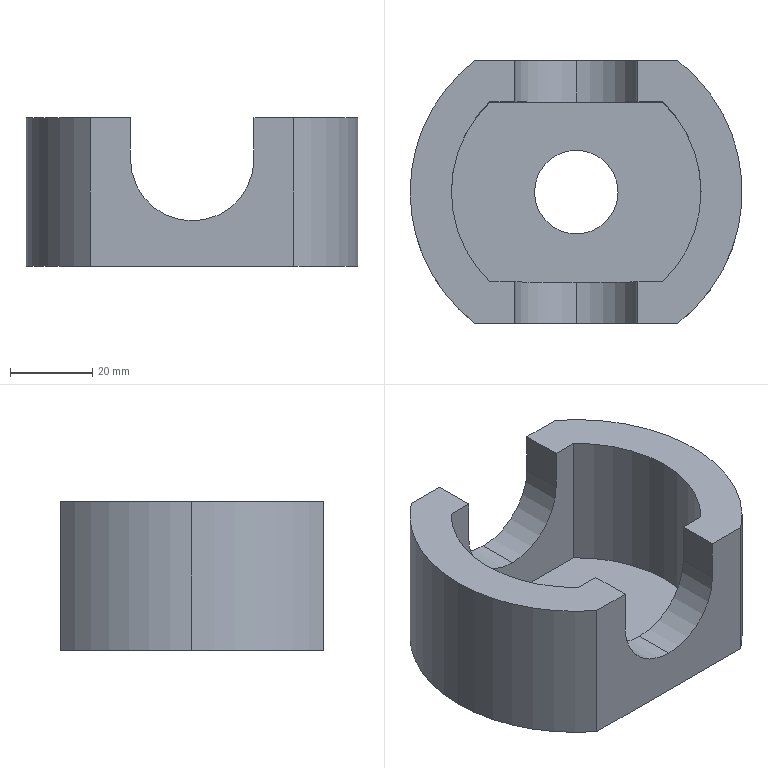Part | SolidWorks | features BaseBody 1 | 1 solid | 24 faces | box 80.6 x 63.7 x 36 mm | volume 68001 mm3 | cylinder 12 | plane 12 | commonest cylinder face diameters 30 x4 60.6 x3 80.6 x3 20.3 x2
STEP:
#1=CARTESIAN_POINT('',(2.562,-19.084,26.));
#2=VERTEX_POINT('',#1);
#3=CARTESIAN_POINT('',(-12.438,-19.084,11.));
#4=VERTEX_POINT('',#3);
#5=CARTESIAN_POINT('',(-12.438,-19.084,26.));
#6=DIRECTION('',(0.,1.,0.));
#7=DIRECTION('',(0.,0.,1.));
#8=AXIS2_PLACEMENT_3D('',#5,#6,#7);
#9=CIRCLE('',#8,15.);
#10=EDGE_CURVE('',#2,#4,#9,.T.);
#11=ORIENTED_EDGE('',*,*,#10,.T.);
#12=CARTESIAN_POINT('',(-12.438,-29.084,11.));
#13=VERTEX_POINT('',#12);
#14=CARTESIAN_POINT('',(-12.438,34.616,11.));
#15=DIRECTION('',(0.,-1.,0.));
#16=VECTOR('',#15,1000.);
#17=LINE('',#14,#16);
#18=EDGE_CURVE('',#4,#13,#17,.T.);
#19=ORIENTED_EDGE('',*,*,#18,.T.);
#20=CARTESIAN_POINT('',(2.562,-29.084,26.));
#21=VERTEX_POINT('',#20);
#22=CARTESIAN_POINT('',(-12.438,-29.084,26.));
#23=DIRECTION('',(0.,-1.,0.));
#24=DIRECTION('',(0.,0.,-1.));
#25=AXIS2_PLACEMENT_3D('',#22,#23,#24);
#26=CIRCLE('',#25,15.);
#27=EDGE_CURVE('',#13,#21,#26,.T.);
#28=ORIENTED_EDGE('',*,*,#27,.T.);
#29=CARTESIAN_POINT('',(2.562,34.616,26.));
#30=DIRECTION('',(0.,-1.,0.));
#31=VECTOR('',#30,1000.);
#32=LINE('',#29,#31);
#33=EDGE_CURVE('',#2,#21,#32,.T.);
#34=ORIENTED_EDGE('',*,*,#33,.F.);
#35=EDGE_LOOP('',(#11,#19,#28,#34));
#36=FACE_OUTER_BOUND('',#35,.T.);
#37=CARTESIAN_POINT('',(-12.438,34.616,26.));
#38=DIRECTION('',(0.,-1.,0.));
#39=DIRECTION('',(0.,0.,-1.));
#40=AXIS2_PLACEMENT_3D('',#37,#38,#39);
#41=CYLINDRICAL_SURFACE('',#40,15.);
#42=ADVANCED_FACE('',(#36),#41,.F.);
#43=CARTESIAN_POINT('',(-12.438,34.616,11.));
#44=VERTEX_POINT('',#43);
#45=CARTESIAN_POINT('',(2.562,34.616,26.));
#46=VERTEX_POINT('',#45);
#47=CARTESIAN_POINT('',(-12.438,34.616,26.));
#48=DIRECTION('',(0.,-1.,0.));
#49=DIRECTION('',(0.,0.,-1.));
#50=AXIS2_PLACEMENT_3D('',#47,#48,#49);
#51=CIRCLE('',#50,15.);
#52=EDGE_CURVE('',#44,#46,#51,.T.);
#53=ORIENTED_EDGE('',*,*,#52,.F.);
#54=CARTESIAN_POINT('',(-12.438,24.616,11.));
#55=VERTEX_POINT('',#54);
#56=CARTESIAN_POINT('',(-12.438,34.616,11.));
#57=DIRECTION('',(0.,-1.,0.));
#58=VECTOR('',#57,1000.);
#59=LINE('',#56,#58);
#60=EDGE_CURVE('',#44,#55,#59,.T.);
#61=ORIENTED_EDGE('',*,*,#60,.T.);
#62=CARTESIAN_POINT('',(2.562,24.616,26.));
#63=VERTEX_POINT('',#62);
#64=CARTESIAN_POINT('',(-12.438,24.616,26.));
#65=DIRECTION('',(0.,-1.,0.));
#66=DIRECTION('',(0.,0.,-1.));
#67=AXIS2_PLACEMENT_3D('',#64,#65,#66);
#68=CIRCLE('',#67,15.);
#69=EDGE_CURVE('',#55,#63,#68,.T.);
#70=ORIENTED_EDGE('',*,*,#69,.T.);
#71=CARTESIAN_POINT('',(2.562,34.616,26.));
#72=DIRECTION('',(0.,-1.,0.));
#73=VECTOR('',#72,1000.);
#74=LINE('',#71,#73);
#75=EDGE_CURVE('',#46,#63,#74,.T.);
#76=ORIENTED_EDGE('',*,*,#75,.F.);
#77=EDGE_LOOP('',(#53,#61,#70,#76));
#78=FACE_OUTER_BOUND('',#77,.T.);
#79=CARTESIAN_POINT('',(-12.438,34.616,26.));
#80=DIRECTION('',(0.,-1.,0.));
#81=DIRECTION('',(0.,0.,-1.));
#82=AXIS2_PLACEMENT_3D('',#79,#80,#81);
#83=CYLINDRICAL_SURFACE('',#82,15.);
#84=ADVANCED_FACE('',(#78),#83,.F.);
#85=CARTESIAN_POINT('',(-33.43,24.616,36.));
#86=VERTEX_POINT('',#85);
#87=CARTESIAN_POINT('',(-42.738,2.766,36.));
#88=VERTEX_POINT('',#87);
#89=CARTESIAN_POINT('',(-12.438,2.766,36.));
#90=DIRECTION('',(0.,0.,1.));
#91=DIRECTION('',(1.,0.,0.));
#92=AXIS2_PLACEMENT_3D('',#89,#90,#91);
#93=CIRCLE('',#92,30.3);
#94=EDGE_CURVE('',#86,#88,#93,.T.);
#95=ORIENTED_EDGE('',*,*,#94,.T.);
#96=CARTESIAN_POINT('',(-42.738,2.766,2.));
#97=VERTEX_POINT('',#96);
#98=CARTESIAN_POINT('',(-42.738,2.766,36.));
#99=DIRECTION('',(0.,0.,-1.));
#100=VECTOR('',#99,1000.);
#101=LINE('',#98,#100);
#102=EDGE_CURVE('',#88,#97,#101,.T.);
#103=ORIENTED_EDGE('',*,*,#102,.T.);
#104=CARTESIAN_POINT('',(-33.43,24.616,2.));
#105=VERTEX_POINT('',#104);
#106=CARTESIAN_POINT('',(-12.438,2.766,2.));
#107=DIRECTION('',(0.,0.,1.));
#108=DIRECTION('',(1.,0.,0.));
#109=AXIS2_PLACEMENT_3D('',#106,#107,#108);
#110=CIRCLE('',#109,30.3);
#111=EDGE_CURVE('',#105,#97,#110,.T.);
#112=ORIENTED_EDGE('',*,*,#111,.F.);
#113=CARTESIAN_POINT('',(-33.43,24.616,36.));
#114=DIRECTION('',(0.,0.,-1.));
#115=VECTOR('',#114,1000.);
#116=LINE('',#113,#115);
#117=EDGE_CURVE('',#86,#105,#116,.T.);
#118=ORIENTED_EDGE('',*,*,#117,.F.);
#119=EDGE_LOOP('',(#95,#103,#112,#118));
#120=FACE_OUTER_BOUND('',#119,.T.);
#121=CARTESIAN_POINT('',(-12.438,2.766,36.));
#122=DIRECTION('',(0.,0.,-1.));
#123=DIRECTION('',(-1.,0.,0.));
#124=AXIS2_PLACEMENT_3D('',#121,#122,#123);
#125=CYLINDRICAL_SURFACE('',#124,30.3);
#126=ADVANCED_FACE('',(#120),#125,.F.);
#127=CARTESIAN_POINT('',(-52.738,2.766,36.));
#128=VERTEX_POINT('',#127);
#129=CARTESIAN_POINT('',(-37.13,-29.084,36.));
#130=VERTEX_POINT('',#129);
#131=CARTESIAN_POINT('',(-12.438,2.766,36.));
#132=DIRECTION('',(0.,0.,1.));
#133=DIRECTION('',(1.,0.,0.));
#134=AXIS2_PLACEMENT_3D('',#131,#132,#133);
#135=CIRCLE('',#134,40.3);
#136=EDGE_CURVE('',#128,#130,#135,.T.);
#137=ORIENTED_EDGE('',*,*,#136,.F.);
#138=CARTESIAN_POINT('',(-52.738,2.766,0.));
#139=VERTEX_POINT('',#138);
#140=CARTESIAN_POINT('',(-52.738,2.766,36.));
#141=DIRECTION('',(0.,0.,-1.));
#142=VECTOR('',#141,1000.);
#143=LINE('',#140,#142);
#144=EDGE_CURVE('',#128,#139,#143,.T.);
#145=ORIENTED_EDGE('',*,*,#144,.T.);
#146=CARTESIAN_POINT('',(-37.13,-29.084,0.));
#147=VERTEX_POINT('',#146);
#148=CARTESIAN_POINT('',(-12.438,2.766,0.));
#149=DIRECTION('',(0.,0.,1.));
#150=DIRECTION('',(1.,0.,0.));
#151=AXIS2_PLACEMENT_3D('',#148,#149,#150);
#152=CIRCLE('',#151,40.3);
#153=EDGE_CURVE('',#139,#147,#152,.T.);
#154=ORIENTED_EDGE('',*,*,#153,.T.);
#155=CARTESIAN_POINT('',(-37.13,-29.084,36.));
#156=DIRECTION('',(0.,0.,-1.));
#157=VECTOR('',#156,1000.);
#158=LINE('',#155,#157);
#159=EDGE_CURVE('',#130,#147,#158,.T.);
#160=ORIENTED_EDGE('',*,*,#159,.F.);
#161=EDGE_LOOP('',(#137,#145,#154,#160));
#162=FACE_OUTER_BOUND('',#161,.T.);
#163=CARTESIAN_POINT('',(-12.438,2.766,36.));
#164=DIRECTION('',(0.,0.,-1.));
#165=DIRECTION('',(-1.,0.,0.));
#166=AXIS2_PLACEMENT_3D('',#163,#164,#165);
#167=CYLINDRICAL_SURFACE('',#166,40.3);
#168=ADVANCED_FACE('',(#162),#167,.T.);
#169=CARTESIAN_POINT('',(-22.588,2.766,0.));
#170=VERTEX_POINT('',#169);
#171=CARTESIAN_POINT('',(-2.288,2.766,0.));
#172=VERTEX_POINT('',#171);
#173=CARTESIAN_POINT('',(-12.438,2.766,0.));
#174=DIRECTION('',(0.,0.,1.));
#175=DIRECTION('',(1.,0.,0.));
#176=AXIS2_PLACEMENT_3D('',#173,#174,#175);
#177=CIRCLE('',#176,10.15);
#178=EDGE_CURVE('',#170,#172,#177,.T.);
#179=ORIENTED_EDGE('',*,*,#178,.F.);
#180=CARTESIAN_POINT('',(-22.588,2.766,2.));
#181=VERTEX_POINT('',#180);
#182=CARTESIAN_POINT('',(-22.588,2.766,10.));
#183=DIRECTION('',(0.,0.,1.));
#184=VECTOR('',#183,1000.);
#185=LINE('',#182,#184);
#186=EDGE_CURVE('',#170,#181,#185,.T.);
#187=ORIENTED_EDGE('',*,*,#186,.T.);
#188=CARTESIAN_POINT('',(-2.288,2.766,2.));
#189=VERTEX_POINT('',#188);
#190=CARTESIAN_POINT('',(-12.438,2.766,2.));
#191=DIRECTION('',(0.,0.,-1.));
#192=DIRECTION('',(1.,0.,0.));
#193=AXIS2_PLACEMENT_3D('',#190,#191,#192);
#194=CIRCLE('',#193,10.15);
#195=EDGE_CURVE('',#189,#181,#194,.T.);
#196=ORIENTED_EDGE('',*,*,#195,.F.);
#197=CARTESIAN_POINT('',(-2.288,2.766,10.));
#198=DIRECTION('',(0.,0.,1.));
#199=VECTOR('',#198,1000.);
#200=LINE('',#197,#199);
#201=EDGE_CURVE('',#172,#189,#200,.T.);
#202=ORIENTED_EDGE('',*,*,#201,.F.);
#203=EDGE_LOOP('',(#179,#187,#196,#202));
#204=FACE_OUTER_BOUND('',#203,.T.);
#205=CARTESIAN_POINT('',(-12.438,2.766,10.));
#206=DIRECTION('',(0.,0.,1.));
#207=DIRECTION('',(1.,0.,0.));
#208=AXIS2_PLACEMENT_3D('',#205,#206,#207);
#209=CYLINDRICAL_SURFACE('',#208,10.15);
#210=ADVANCED_FACE('',(#204),#209,.F.);
#211=ORIENTED_EDGE('',*,*,#195,.T.);
#212=CARTESIAN_POINT('',(-12.438,2.766,2.));
#213=DIRECTION('',(0.,0.,-1.));
#214=DIRECTION('',(1.,0.,0.));
#215=AXIS2_PLACEMENT_3D('',#212,#213,#214);
#216=CIRCLE('',#215,10.15);
#217=EDGE_CURVE('',#181,#189,#216,.T.);
#218=ORIENTED_EDGE('',*,*,#217,.T.);
#219=EDGE_LOOP('',(#211,#218));
#220=FACE_BOUND('',#219,.T.);
#221=CARTESIAN_POINT('',(8.554,24.616,2.));
#222=VERTEX_POINT('',#221);
#223=CARTESIAN_POINT('',(8.554,24.616,2.));
#224=DIRECTION('',(-1.,0.,0.));
#225=VECTOR('',#224,1000.);
#226=LINE('',#223,#225);
#227=EDGE_CURVE('',#222,#105,#226,.T.);
#228=ORIENTED_EDGE('',*,*,#227,.T.);
#229=ORIENTED_EDGE('',*,*,#111,.T.);
#230=CARTESIAN_POINT('',(-33.43,-19.084,2.));
#231=VERTEX_POINT('',#230);
#232=CARTESIAN_POINT('',(-12.438,2.766,2.));
#233=DIRECTION('',(0.,0.,1.));
#234=DIRECTION('',(1.,0.,0.));
#235=AXIS2_PLACEMENT_3D('',#232,#233,#234);
#236=CIRCLE('',#235,30.3);
#237=EDGE_CURVE('',#97,#231,#236,.T.);
#238=ORIENTED_EDGE('',*,*,#237,.T.);
#239=CARTESIAN_POINT('',(8.554,-19.084,2.));
#240=VERTEX_POINT('',#239);
#241=CARTESIAN_POINT('',(-33.43,-19.084,2.));
#242=DIRECTION('',(1.,0.,0.));
#243=VECTOR('',#242,1000.);
#244=LINE('',#241,#243);
#245=EDGE_CURVE('',#231,#240,#244,.T.);
#246=ORIENTED_EDGE('',*,*,#245,.T.);
#247=CARTESIAN_POINT('',(-12.438,2.766,2.));
#248=DIRECTION('',(0.,0.,1.));
#249=DIRECTION('',(1.,0.,0.));
#250=AXIS2_PLACEMENT_3D('',#247,#248,#249);
#251=CIRCLE('',#250,30.3);
#252=EDGE_CURVE('',#240,#222,#251,.T.);
#253=ORIENTED_EDGE('',*,*,#252,.T.);
#254=EDGE_LOOP('',(#228,#229,#238,#246,#253));
#255=FACE_OUTER_BOUND('',#254,.T.);
#256=CARTESIAN_POINT('',(-12.438,2.766,2.));
#257=DIRECTION('',(0.,0.,1.));
#258=DIRECTION('',(1.,0.,0.));
#259=AXIS2_PLACEMENT_3D('',#256,#257,#258);
#260=PLANE('',#259);
#261=ADVANCED_FACE('',(#220,#255),#260,.T.);
#262=CARTESIAN_POINT('',(2.562,-29.084,36.));
#263=VERTEX_POINT('',#262);
#264=CARTESIAN_POINT('',(2.562,-19.084,36.));
#265=VERTEX_POINT('',#264);
#266=CARTESIAN_POINT('',(2.562,2.766,36.));
#267=DIRECTION('',(0.,1.,0.));
#268=VECTOR('',#267,1000.);
#269=LINE('',#266,#268);
#270=EDGE_CURVE('',#263,#265,#269,.T.);
#271=ORIENTED_EDGE('',*,*,#270,.T.);
#272=CARTESIAN_POINT('',(2.562,-19.084,36.));
#273=DIRECTION('',(0.,0.,-1.));
#274=VECTOR('',#273,1000.);
#275=LINE('',#272,#274);
#276=EDGE_CURVE('',#265,#2,#275,.T.);
#277=ORIENTED_EDGE('',*,*,#276,.T.);
#278=ORIENTED_EDGE('',*,*,#33,.T.);
#279=CARTESIAN_POINT('',(2.562,-29.084,49.375));
#280=DIRECTION('',(0.,0.,1.));
#281=VECTOR('',#280,1000.);
#282=LINE('',#279,#281);
#283=EDGE_CURVE('',#21,#263,#282,.T.);
#284=ORIENTED_EDGE('',*,*,#283,.T.);
#285=EDGE_LOOP('',(#271,#277,#278,#284));
#286=FACE_OUTER_BOUND('',#285,.T.);
#287=CARTESIAN_POINT('',(2.562,34.616,49.375));
#288=DIRECTION('',(1.,0.,0.));
#289=DIRECTION('',(0.,0.,-1.));
#290=AXIS2_PLACEMENT_3D('',#287,#288,#289);
#291=PLANE('',#290);
#292=ADVANCED_FACE('',(#286),#291,.F.);
#293=CARTESIAN_POINT('',(-27.438,-19.084,36.));
#294=VERTEX_POINT('',#293);
#295=CARTESIAN_POINT('',(-27.438,-29.084,36.));
#296=VERTEX_POINT('',#295);
#297=CARTESIAN_POINT('',(-27.438,2.766,36.));
#298=DIRECTION('',(0.,-1.,0.));
#299=VECTOR('',#298,1000.);
#300=LINE('',#297,#299);
#301=EDGE_CURVE('',#294,#296,#300,.T.);
#302=ORIENTED_EDGE('',*,*,#301,.T.);
#303=CARTESIAN_POINT('',(-27.438,-29.084,26.));
#304=VERTEX_POINT('',#303);
#305=CARTESIAN_POINT('',(-27.438,-29.084,49.375));
#306=DIRECTION('',(0.,0.,-1.));
#307=VECTOR('',#306,1000.);
#308=LINE('',#305,#307);
#309=EDGE_CURVE('',#296,#304,#308,.T.);
#310=ORIENTED_EDGE('',*,*,#309,.T.);
#311=CARTESIAN_POINT('',(-27.438,-19.084,26.));
#312=VERTEX_POINT('',#311);
#313=CARTESIAN_POINT('',(-27.438,34.616,26.));
#314=DIRECTION('',(0.,-1.,0.));
#315=VECTOR('',#314,1000.);
#316=LINE('',#313,#315);
#317=EDGE_CURVE('',#312,#304,#316,.T.);
#318=ORIENTED_EDGE('',*,*,#317,.F.);
#319=CARTESIAN_POINT('',(-27.438,-19.084,36.));
#320=DIRECTION('',(0.,0.,1.));
#321=VECTOR('',#320,1000.);
#322=LINE('',#319,#321);
#323=EDGE_CURVE('',#312,#294,#322,.T.);
#324=ORIENTED_EDGE('',*,*,#323,.T.);
#325=EDGE_LOOP('',(#302,#310,#318,#324));
#326=FACE_OUTER_BOUND('',#325,.T.);
#327=CARTESIAN_POINT('',(-27.438,34.616,49.375));
#328=DIRECTION('',(-1.,0.,0.));
#329=DIRECTION('',(0.,0.,1.));
#330=AXIS2_PLACEMENT_3D('',#327,#328,#329);
#331=PLANE('',#330);
#332=ADVANCED_FACE('',(#326),#331,.F.);
#333=CARTESIAN_POINT('',(-27.438,34.616,36.));
#334=VERTEX_POINT('',#333);
#335=CARTESIAN_POINT('',(-27.438,24.616,36.));
#336=VERTEX_POINT('',#335);
#337=CARTESIAN_POINT('',(-27.438,2.766,36.));
#338=DIRECTION('',(0.,-1.,0.));
#339=VECTOR('',#338,1000.);
#340=LINE('',#337,#339);
#341=EDGE_CURVE('',#334,#336,#340,.T.);
#342=ORIENTED_EDGE('',*,*,#341,.T.);
#343=CARTESIAN_POINT('',(-27.438,24.616,26.));
#344=VERTEX_POINT('',#343);
#345=CARTESIAN_POINT('',(-27.438,24.616,36.));
#346=DIRECTION('',(0.,0.,-1.));
#347=VECTOR('',#346,1000.);
#348=LINE('',#345,#347);
#349=EDGE_CURVE('',#336,#344,#348,.T.);
#350=ORIENTED_EDGE('',*,*,#349,.T.);
#351=CARTESIAN_POINT('',(-27.438,34.616,26.));
#352=VERTEX_POINT('',#351);
#353=CARTESIAN_POINT('',(-27.438,34.616,26.));
#354=DIRECTION('',(0.,-1.,0.));
#355=VECTOR('',#354,1000.);
#356=LINE('',#353,#355);
#357=EDGE_CURVE('',#352,#344,#356,.T.);
#358=ORIENTED_EDGE('',*,*,#357,.F.);
#359=CARTESIAN_POINT('',(-27.438,34.616,49.375));
#360=DIRECTION('',(0.,0.,-1.));
#361=VECTOR('',#360,1000.);
#362=LINE('',#359,#361);
#363=EDGE_CURVE('',#334,#352,#362,.T.);
#364=ORIENTED_EDGE('',*,*,#363,.F.);
#365=EDGE_LOOP('',(#342,#350,#358,#364));
#366=FACE_OUTER_BOUND('',#365,.T.);
#367=CARTESIAN_POINT('',(-27.438,34.616,49.375));
#368=DIRECTION('',(-1.,0.,0.));
#369=DIRECTION('',(0.,0.,1.));
#370=AXIS2_PLACEMENT_3D('',#367,#368,#369);
#371=PLANE('',#370);
#372=ADVANCED_FACE('',(#366),#371,.F.);
#373=CARTESIAN_POINT('',(2.562,24.616,36.));
#374=VERTEX_POINT('',#373);
#375=CARTESIAN_POINT('',(2.562,34.616,36.));
#376=VERTEX_POINT('',#375);
#377=CARTESIAN_POINT('',(2.562,2.766,36.));
#378=DIRECTION('',(0.,1.,0.));
#379=VECTOR('',#378,1000.);
#380=LINE('',#377,#379);
#381=EDGE_CURVE('',#374,#376,#380,.T.);
#382=ORIENTED_EDGE('',*,*,#381,.T.);
#383=CARTESIAN_POINT('',(2.562,34.616,49.375));
#384=DIRECTION('',(0.,0.,1.));
#385=VECTOR('',#384,1000.);
#386=LINE('',#383,#385);
#387=EDGE_CURVE('',#46,#376,#386,.T.);
#388=ORIENTED_EDGE('',*,*,#387,.F.);
#389=ORIENTED_EDGE('',*,*,#75,.T.);
#390=CARTESIAN_POINT('',(2.562,24.616,36.));
#391=DIRECTION('',(0.,0.,1.));
#392=VECTOR('',#391,1000.);
#393=LINE('',#390,#392);
#394=EDGE_CURVE('',#63,#374,#393,.T.);
#395=ORIENTED_EDGE('',*,*,#394,.T.);
#396=EDGE_LOOP('',(#382,#388,#389,#395));
#397=FACE_OUTER_BOUND('',#396,.T.);
#398=CARTESIAN_POINT('',(2.562,34.616,49.375));
#399=DIRECTION('',(1.,0.,0.));
#400=DIRECTION('',(0.,0.,-1.));
#401=AXIS2_PLACEMENT_3D('',#398,#399,#400);
#402=PLANE('',#401);
#403=ADVANCED_FACE('',(#397),#402,.F.);
#404=ORIENTED_EDGE('',*,*,#349,.F.);
#405=CARTESIAN_POINT('',(-37.13,24.616,36.));
#406=DIRECTION('',(-1.,0.,0.));
#407=VECTOR('',#406,1000.);
#408=LINE('',#405,#407);
#409=EDGE_CURVE('',#336,#86,#408,.T.);
#410=ORIENTED_EDGE('',*,*,#409,.T.);
#411=ORIENTED_EDGE('',*,*,#117,.T.);
#412=ORIENTED_EDGE('',*,*,#227,.F.);
#413=CARTESIAN_POINT('',(8.554,24.616,36.));
#414=VERTEX_POINT('',#413);
#415=CARTESIAN_POINT('',(8.554,24.616,36.));
#416=DIRECTION('',(0.,0.,-1.));
#417=VECTOR('',#416,1000.);
#418=LINE('',#415,#417);
#419=EDGE_CURVE('',#414,#222,#418,.T.);
#420=ORIENTED_EDGE('',*,*,#419,.F.);
#421=CARTESIAN_POINT('',(-37.13,24.616,36.));
#422=DIRECTION('',(-1.,0.,0.));
#423=VECTOR('',#422,1000.);
#424=LINE('',#421,#423);
#425=EDGE_CURVE('',#414,#374,#424,.T.);
#426=ORIENTED_EDGE('',*,*,#425,.T.);
#427=ORIENTED_EDGE('',*,*,#394,.F.);
#428=ORIENTED_EDGE('',*,*,#69,.F.);
#429=CARTESIAN_POINT('',(-12.438,24.616,26.));
#430=DIRECTION('',(0.,-1.,0.));
#431=DIRECTION('',(0.,0.,-1.));
#432=AXIS2_PLACEMENT_3D('',#429,#430,#431);
#433=CIRCLE('',#432,15.);
#434=EDGE_CURVE('',#344,#55,#433,.T.);
#435=ORIENTED_EDGE('',*,*,#434,.F.);
#436=EDGE_LOOP('',(#404,#410,#411,#412,#420,#426,#427,#428,#435));
#437=FACE_OUTER_BOUND('',#436,.T.);
#438=CARTESIAN_POINT('',(-37.13,24.616,36.));
#439=DIRECTION('',(0.,-1.,0.));
#440=DIRECTION('',(0.,0.,-1.));
#441=AXIS2_PLACEMENT_3D('',#438,#439,#440);
#442=PLANE('',#441);
#443=ADVANCED_FACE('',(#437),#442,.T.);
#444=ORIENTED_EDGE('',*,*,#419,.T.);
#445=ORIENTED_EDGE('',*,*,#252,.F.);
#446=CARTESIAN_POINT('',(8.554,-19.084,36.));
#447=VERTEX_POINT('',#446);
#448=CARTESIAN_POINT('',(8.554,-19.084,36.));
#449=DIRECTION('',(0.,0.,-1.));
#450=VECTOR('',#449,1000.);
#451=LINE('',#448,#450);
#452=EDGE_CURVE('',#447,#240,#451,.T.);
#453=ORIENTED_EDGE('',*,*,#452,.F.);
#454=CARTESIAN_POINT('',(-12.438,2.766,36.));
#455=DIRECTION('',(0.,0.,1.));
#456=DIRECTION('',(1.,0.,0.));
#457=AXIS2_PLACEMENT_3D('',#454,#455,#456);
#458=CIRCLE('',#457,30.3);
#459=EDGE_CURVE('',#447,#414,#458,.T.);
#460=ORIENTED_EDGE('',*,*,#459,.T.);
#461=EDGE_LOOP('',(#444,#445,#453,#460));
#462=FACE_OUTER_BOUND('',#461,.T.);
#463=CARTESIAN_POINT('',(-12.438,2.766,36.));
#464=DIRECTION('',(0.,0.,-1.));
#465=DIRECTION('',(-1.,0.,0.));
#466=AXIS2_PLACEMENT_3D('',#463,#464,#465);
#467=CYLINDRICAL_SURFACE('',#466,30.3);
#468=ADVANCED_FACE('',(#462),#467,.F.);
#469=ORIENTED_EDGE('',*,*,#323,.F.);
#470=CARTESIAN_POINT('',(-12.438,-19.084,26.));
#471=DIRECTION('',(0.,1.,0.));
#472=DIRECTION('',(0.,0.,1.));
#473=AXIS2_PLACEMENT_3D('',#470,#471,#472);
#474=CIRCLE('',#473,15.);
#475=EDGE_CURVE('',#4,#312,#474,.T.);
#476=ORIENTED_EDGE('',*,*,#475,.F.);
#477=ORIENTED_EDGE('',*,*,#10,.F.);
#478=ORIENTED_EDGE('',*,*,#276,.F.);
#479=CARTESIAN_POINT('',(-37.13,-19.084,36.));
#480=DIRECTION('',(1.,0.,0.));
#481=VECTOR('',#480,1000.);
#482=LINE('',#479,#481);
#483=EDGE_CURVE('',#265,#447,#482,.T.);
#484=ORIENTED_EDGE('',*,*,#483,.T.);
#485=ORIENTED_EDGE('',*,*,#452,.T.);
#486=ORIENTED_EDGE('',*,*,#245,.F.);
#487=CARTESIAN_POINT('',(-33.43,-19.084,36.));
#488=VERTEX_POINT('',#487);
#489=CARTESIAN_POINT('',(-33.43,-19.084,36.));
#490=DIRECTION('',(0.,0.,-1.));
#491=VECTOR('',#490,1000.);
#492=LINE('',#489,#491);
#493=EDGE_CURVE('',#488,#231,#492,.T.);
#494=ORIENTED_EDGE('',*,*,#493,.F.);
#495=CARTESIAN_POINT('',(-37.13,-19.084,36.));
#496=DIRECTION('',(1.,0.,0.));
#497=VECTOR('',#496,1000.);
#498=LINE('',#495,#497);
#499=EDGE_CURVE('',#488,#294,#498,.T.);
#500=ORIENTED_EDGE('',*,*,#499,.T.);
#501=EDGE_LOOP('',(#469,#476,#477,#478,#484,#485,#486,#494,#500));
#502=FACE_OUTER_BOUND('',#501,.T.);
#503=CARTESIAN_POINT('',(-37.13,-19.084,36.));
#504=DIRECTION('',(0.,1.,0.));
#505=DIRECTION('',(1.,0.,0.));
#506=AXIS2_PLACEMENT_3D('',#503,#504,#505);
#507=PLANE('',#506);
#508=ADVANCED_FACE('',(#502),#507,.T.);
#509=CARTESIAN_POINT('',(-12.438,2.766,0.));
#510=DIRECTION('',(0.,0.,1.));
#511=DIRECTION('',(1.,0.,0.));
#512=AXIS2_PLACEMENT_3D('',#509,#510,#511);
#513=CIRCLE('',#512,10.15);
#514=EDGE_CURVE('',#172,#170,#513,.T.);
#515=ORIENTED_EDGE('',*,*,#514,.T.);
#516=ORIENTED_EDGE('',*,*,#178,.T.);
#517=EDGE_LOOP('',(#515,#516));
#518=FACE_BOUND('',#517,.T.);
#519=CARTESIAN_POINT('',(-37.13,34.616,0.));
#520=VERTEX_POINT('',#519);
#521=CARTESIAN_POINT('',(-12.438,2.766,0.));
#522=DIRECTION('',(0.,0.,1.));
#523=DIRECTION('',(1.,0.,0.));
#524=AXIS2_PLACEMENT_3D('',#521,#522,#523);
#525=CIRCLE('',#524,40.3);
#526=EDGE_CURVE('',#520,#139,#525,.T.);
#527=ORIENTED_EDGE('',*,*,#526,.F.);
#528=CARTESIAN_POINT('',(12.253,34.616,0.));
#529=VERTEX_POINT('',#528);
#530=CARTESIAN_POINT('',(-37.13,34.616,0.));
#531=DIRECTION('',(-1.,0.,0.));
#532=VECTOR('',#531,1000.);
#533=LINE('',#530,#532);
#534=EDGE_CURVE('',#529,#520,#533,.T.);
#535=ORIENTED_EDGE('',*,*,#534,.F.);
#536=CARTESIAN_POINT('',(12.253,-29.084,0.));
#537=VERTEX_POINT('',#536);
#538=CARTESIAN_POINT('',(-12.438,2.766,0.));
#539=DIRECTION('',(0.,0.,1.));
#540=DIRECTION('',(1.,0.,0.));
#541=AXIS2_PLACEMENT_3D('',#538,#539,#540);
#542=CIRCLE('',#541,40.3);
#543=EDGE_CURVE('',#537,#529,#542,.T.);
#544=ORIENTED_EDGE('',*,*,#543,.F.);
#545=CARTESIAN_POINT('',(-37.13,-29.084,0.));
#546=DIRECTION('',(1.,0.,0.));
#547=VECTOR('',#546,1000.);
#548=LINE('',#545,#547);
#549=EDGE_CURVE('',#147,#537,#548,.T.);
#550=ORIENTED_EDGE('',*,*,#549,.F.);
#551=ORIENTED_EDGE('',*,*,#153,.F.);
#552=EDGE_LOOP('',(#527,#535,#544,#550,#551));
#553=FACE_OUTER_BOUND('',#552,.T.);
#554=CARTESIAN_POINT('',(-12.438,2.766,0.));
#555=DIRECTION('',(0.,0.,1.));
#556=DIRECTION('',(1.,0.,0.));
#557=AXIS2_PLACEMENT_3D('',#554,#555,#556);
#558=PLANE('',#557);
#559=ADVANCED_FACE('',(#518,#553),#558,.F.);
#560=ORIENTED_EDGE('',*,*,#270,.F.);
#561=CARTESIAN_POINT('',(12.253,-29.084,36.));
#562=VERTEX_POINT('',#561);
#563=CARTESIAN_POINT('',(-37.13,-29.084,36.));
#564=DIRECTION('',(1.,0.,0.));
#565=VECTOR('',#564,1000.);
#566=LINE('',#563,#565);
#567=EDGE_CURVE('',#263,#562,#566,.T.);
#568=ORIENTED_EDGE('',*,*,#567,.T.);
#569=CARTESIAN_POINT('',(12.253,34.616,36.));
#570=VERTEX_POINT('',#569);
#571=CARTESIAN_POINT('',(-12.438,2.766,36.));
#572=DIRECTION('',(0.,0.,1.));
#573=DIRECTION('',(1.,0.,0.));
#574=AXIS2_PLACEMENT_3D('',#571,#572,#573);
#575=CIRCLE('',#574,40.3);
#576=EDGE_CURVE('',#562,#570,#575,.T.);
#577=ORIENTED_EDGE('',*,*,#576,.T.);
#578=CARTESIAN_POINT('',(-37.13,34.616,36.));
#579=DIRECTION('',(-1.,0.,0.));
#580=VECTOR('',#579,1000.);
#581=LINE('',#578,#580);
#582=EDGE_CURVE('',#570,#376,#581,.T.);
#583=ORIENTED_EDGE('',*,*,#582,.T.);
#584=ORIENTED_EDGE('',*,*,#381,.F.);
#585=ORIENTED_EDGE('',*,*,#425,.F.);
#586=ORIENTED_EDGE('',*,*,#459,.F.);
#587=ORIENTED_EDGE('',*,*,#483,.F.);
#588=EDGE_LOOP('',(#560,#568,#577,#583,#584,#585,#586,#587));
#589=FACE_OUTER_BOUND('',#588,.T.);
#590=CARTESIAN_POINT('',(-12.438,2.766,36.));
#591=DIRECTION('',(0.,0.,1.));
#592=DIRECTION('',(1.,0.,0.));
#593=AXIS2_PLACEMENT_3D('',#590,#591,#592);
#594=PLANE('',#593);
#595=ADVANCED_FACE('',(#589),#594,.T.);
#596=CARTESIAN_POINT('',(-37.13,34.616,36.));
#597=VERTEX_POINT('',#596);
#598=CARTESIAN_POINT('',(-37.13,34.616,36.));
#599=DIRECTION('',(-1.,0.,0.));
#600=VECTOR('',#599,1000.);
#601=LINE('',#598,#600);
#602=EDGE_CURVE('',#334,#597,#601,.T.);
#603=ORIENTED_EDGE('',*,*,#602,.F.);
#604=ORIENTED_EDGE('',*,*,#363,.T.);
#605=CARTESIAN_POINT('',(-12.438,34.616,26.));
#606=DIRECTION('',(0.,-1.,0.));
#607=DIRECTION('',(0.,0.,-1.));
#608=AXIS2_PLACEMENT_3D('',#605,#606,#607);
#609=CIRCLE('',#608,15.);
#610=EDGE_CURVE('',#352,#44,#609,.T.);
#611=ORIENTED_EDGE('',*,*,#610,.T.);
#612=ORIENTED_EDGE('',*,*,#52,.T.);
#613=ORIENTED_EDGE('',*,*,#387,.T.);
#614=ORIENTED_EDGE('',*,*,#582,.F.);
#615=CARTESIAN_POINT('',(12.253,34.616,36.));
#616=DIRECTION('',(0.,0.,-1.));
#617=VECTOR('',#616,1000.);
#618=LINE('',#615,#617);
#619=EDGE_CURVE('',#570,#529,#618,.T.);
#620=ORIENTED_EDGE('',*,*,#619,.T.);
#621=ORIENTED_EDGE('',*,*,#534,.T.);
#622=CARTESIAN_POINT('',(-37.13,34.616,36.));
#623=DIRECTION('',(0.,0.,-1.));
#624=VECTOR('',#623,1000.);
#625=LINE('',#622,#624);
#626=EDGE_CURVE('',#597,#520,#625,.T.);
#627=ORIENTED_EDGE('',*,*,#626,.F.);
#628=EDGE_LOOP('',(#603,#604,#611,#612,#613,#614,#620,#621,#627));
#629=FACE_OUTER_BOUND('',#628,.T.);
#630=CARTESIAN_POINT('',(-37.13,34.616,36.));
#631=DIRECTION('',(0.,-1.,0.));
#632=DIRECTION('',(0.,0.,-1.));
#633=AXIS2_PLACEMENT_3D('',#630,#631,#632);
#634=PLANE('',#633);
#635=ADVANCED_FACE('',(#629),#634,.F.);
#636=ORIENTED_EDGE('',*,*,#543,.T.);
#637=ORIENTED_EDGE('',*,*,#619,.F.);
#638=ORIENTED_EDGE('',*,*,#576,.F.);
#639=CARTESIAN_POINT('',(12.253,-29.084,36.));
#640=DIRECTION('',(0.,0.,-1.));
#641=VECTOR('',#640,1000.);
#642=LINE('',#639,#641);
#643=EDGE_CURVE('',#562,#537,#642,.T.);
#644=ORIENTED_EDGE('',*,*,#643,.T.);
#645=EDGE_LOOP('',(#636,#637,#638,#644));
#646=FACE_OUTER_BOUND('',#645,.T.);
#647=CARTESIAN_POINT('',(-12.438,2.766,36.));
#648=DIRECTION('',(0.,0.,-1.));
#649=DIRECTION('',(-1.,0.,0.));
#650=AXIS2_PLACEMENT_3D('',#647,#648,#649);
#651=CYLINDRICAL_SURFACE('',#650,40.3);
#652=ADVANCED_FACE('',(#646),#651,.T.);
#653=CARTESIAN_POINT('',(-12.438,-29.084,26.));
#654=DIRECTION('',(0.,-1.,0.));
#655=DIRECTION('',(0.,0.,-1.));
#656=AXIS2_PLACEMENT_3D('',#653,#654,#655);
#657=CIRCLE('',#656,15.);
#658=EDGE_CURVE('',#304,#13,#657,.T.);
#659=ORIENTED_EDGE('',*,*,#658,.F.);
#660=ORIENTED_EDGE('',*,*,#309,.F.);
#661=CARTESIAN_POINT('',(-37.13,-29.084,36.));
#662=DIRECTION('',(1.,0.,0.));
#663=VECTOR('',#662,1000.);
#664=LINE('',#661,#663);
#665=EDGE_CURVE('',#130,#296,#664,.T.);
#666=ORIENTED_EDGE('',*,*,#665,.F.);
#667=ORIENTED_EDGE('',*,*,#159,.T.);
#668=ORIENTED_EDGE('',*,*,#549,.T.);
#669=ORIENTED_EDGE('',*,*,#643,.F.);
#670=ORIENTED_EDGE('',*,*,#567,.F.);
#671=ORIENTED_EDGE('',*,*,#283,.F.);
#672=ORIENTED_EDGE('',*,*,#27,.F.);
#673=EDGE_LOOP('',(#659,#660,#666,#667,#668,#669,#670,#671,#672));
#674=FACE_OUTER_BOUND('',#673,.T.);
#675=CARTESIAN_POINT('',(-37.13,-29.084,36.));
#676=DIRECTION('',(0.,1.,0.));
#677=DIRECTION('',(1.,0.,0.));
#678=AXIS2_PLACEMENT_3D('',#675,#676,#677);
#679=PLANE('',#678);
#680=ADVANCED_FACE('',(#674),#679,.F.);
#681=ORIENTED_EDGE('',*,*,#341,.F.);
#682=ORIENTED_EDGE('',*,*,#602,.T.);
#683=CARTESIAN_POINT('',(-12.438,2.766,36.));
#684=DIRECTION('',(0.,0.,1.));
#685=DIRECTION('',(1.,0.,0.));
#686=AXIS2_PLACEMENT_3D('',#683,#684,#685);
#687=CIRCLE('',#686,40.3);
#688=EDGE_CURVE('',#597,#128,#687,.T.);
#689=ORIENTED_EDGE('',*,*,#688,.T.);
#690=ORIENTED_EDGE('',*,*,#136,.T.);
#691=ORIENTED_EDGE('',*,*,#665,.T.);
#692=ORIENTED_EDGE('',*,*,#301,.F.);
#693=ORIENTED_EDGE('',*,*,#499,.F.);
#694=CARTESIAN_POINT('',(-12.438,2.766,36.));
#695=DIRECTION('',(0.,0.,1.));
#696=DIRECTION('',(1.,0.,0.));
#697=AXIS2_PLACEMENT_3D('',#694,#695,#696);
#698=CIRCLE('',#697,30.3);
#699=EDGE_CURVE('',#88,#488,#698,.T.);
#700=ORIENTED_EDGE('',*,*,#699,.F.);
#701=ORIENTED_EDGE('',*,*,#94,.F.);
#702=ORIENTED_EDGE('',*,*,#409,.F.);
#703=EDGE_LOOP('',(#681,#682,#689,#690,#691,#692,#693,#700,#701,#702));
#704=FACE_OUTER_BOUND('',#703,.T.);
#705=CARTESIAN_POINT('',(-12.438,2.766,36.));
#706=DIRECTION('',(0.,0.,1.));
#707=DIRECTION('',(1.,0.,0.));
#708=AXIS2_PLACEMENT_3D('',#705,#706,#707);
#709=PLANE('',#708);
#710=ADVANCED_FACE('',(#704),#709,.T.);
#711=ORIENTED_EDGE('',*,*,#186,.F.);
#712=ORIENTED_EDGE('',*,*,#514,.F.);
#713=ORIENTED_EDGE('',*,*,#201,.T.);
#714=ORIENTED_EDGE('',*,*,#217,.F.);
#715=EDGE_LOOP('',(#711,#712,#713,#714));
#716=FACE_OUTER_BOUND('',#715,.T.);
#717=CARTESIAN_POINT('',(-12.438,2.766,10.));
#718=DIRECTION('',(0.,0.,1.));
#719=DIRECTION('',(1.,0.,0.));
#720=AXIS2_PLACEMENT_3D('',#717,#718,#719);
#721=CYLINDRICAL_SURFACE('',#720,10.15);
#722=ADVANCED_FACE('',(#716),#721,.F.);
#723=ORIENTED_EDGE('',*,*,#144,.F.);
#724=ORIENTED_EDGE('',*,*,#688,.F.);
#725=ORIENTED_EDGE('',*,*,#626,.T.);
#726=ORIENTED_EDGE('',*,*,#526,.T.);
#727=EDGE_LOOP('',(#723,#724,#725,#726));
#728=FACE_OUTER_BOUND('',#727,.T.);
#729=CARTESIAN_POINT('',(-12.438,2.766,36.));
#730=DIRECTION('',(0.,0.,-1.));
#731=DIRECTION('',(-1.,0.,0.));
#732=AXIS2_PLACEMENT_3D('',#729,#730,#731);
#733=CYLINDRICAL_SURFACE('',#732,40.3);
#734=ADVANCED_FACE('',(#728),#733,.T.);
#735=ORIENTED_EDGE('',*,*,#102,.F.);
#736=ORIENTED_EDGE('',*,*,#699,.T.);
#737=ORIENTED_EDGE('',*,*,#493,.T.);
#738=ORIENTED_EDGE('',*,*,#237,.F.);
#739=EDGE_LOOP('',(#735,#736,#737,#738));
#740=FACE_OUTER_BOUND('',#739,.T.);
#741=CARTESIAN_POINT('',(-12.438,2.766,36.));
#742=DIRECTION('',(0.,0.,-1.));
#743=DIRECTION('',(-1.,0.,0.));
#744=AXIS2_PLACEMENT_3D('',#741,#742,#743);
#745=CYLINDRICAL_SURFACE('',#744,30.3);
#746=ADVANCED_FACE('',(#740),#745,.F.);
#747=ORIENTED_EDGE('',*,*,#60,.F.);
#748=ORIENTED_EDGE('',*,*,#610,.F.);
#749=ORIENTED_EDGE('',*,*,#357,.T.);
#750=ORIENTED_EDGE('',*,*,#434,.T.);
#751=EDGE_LOOP('',(#747,#748,#749,#750));
#752=FACE_OUTER_BOUND('',#751,.T.);
#753=CARTESIAN_POINT('',(-12.438,34.616,26.));
#754=DIRECTION('',(0.,-1.,0.));
#755=DIRECTION('',(0.,0.,-1.));
#756=AXIS2_PLACEMENT_3D('',#753,#754,#755);
#757=CYLINDRICAL_SURFACE('',#756,15.);
#758=ADVANCED_FACE('',(#752),#757,.F.);
#759=ORIENTED_EDGE('',*,*,#18,.F.);
#760=ORIENTED_EDGE('',*,*,#475,.T.);
#761=ORIENTED_EDGE('',*,*,#317,.T.);
#762=ORIENTED_EDGE('',*,*,#658,.T.);
#763=EDGE_LOOP('',(#759,#760,#761,#762));
#764=FACE_OUTER_BOUND('',#763,.T.);
#765=CARTESIAN_POINT('',(-12.438,34.616,26.));
#766=DIRECTION('',(0.,-1.,0.));
#767=DIRECTION('',(0.,0.,-1.));
#768=AXIS2_PLACEMENT_3D('',#765,#766,#767);
#769=CYLINDRICAL_SURFACE('',#768,15.);
#770=ADVANCED_FACE('',(#764),#769,.F.);
#771=CLOSED_SHELL('',(#42,#84,#126,#168,#210,#261,#292,#332,#372,#403,#443,#468,#508,#559,#595,#635,#652,#680,#710,#722,#734,#746,#758,#770));
#772=MANIFOLD_SOLID_BREP('',#771);
#773=CARTESIAN_POINT('',(0.,0.,0.));
#774=DIRECTION('',(0.,0.,1.));
#775=DIRECTION('',(1.,0.,0.));
#776=AXIS2_PLACEMENT_3D('',#773,#774,#775);
#777=(LENGTH_UNIT()NAMED_UNIT(*)SI_UNIT(.MILLI.,.METRE.));
#778=UNCERTAINTY_MEASURE_WITH_UNIT(LENGTH_MEASURE(0.00001),#777,'','');
#779=(NAMED_UNIT(*)PLANE_ANGLE_UNIT()SI_UNIT($,.RADIAN.));
#780=(NAMED_UNIT(*)SI_UNIT($,.STERADIAN.)SOLID_ANGLE_UNIT());
#781=(GEOMETRIC_REPRESENTATION_CONTEXT(3)GLOBAL_UNCERTAINTY_ASSIGNED_CONTEXT((#778))GLOBAL_UNIT_ASSIGNED_CONTEXT((#777,#779,#780))REPRESENTATION_CONTEXT('',''));
#782=ADVANCED_BREP_SHAPE_REPRESENTATION('',(#772,#776),#781);